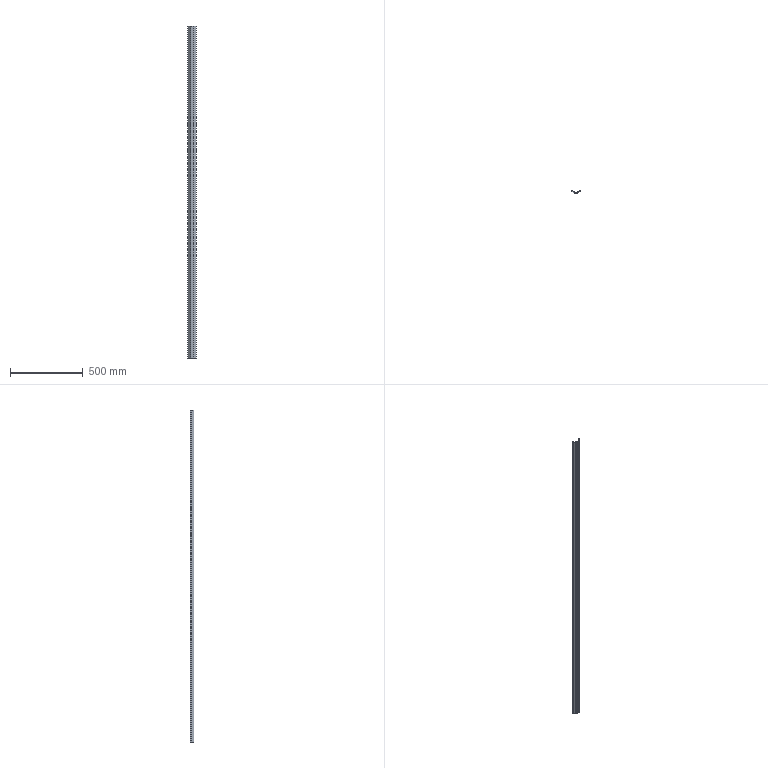Part | SolidWorks | features Extrusion 1 | 1 solid | 40 faces | box 56.572 x 22.358 x 2285 mm | volume 383048 mm3 | plane 37 | cylinder 3 | commonest cylinder face diameters 1 x2 0.5 x1
STEP:
#1=CARTESIAN_POINT('',(6.75,2.,-1142.5));
#2=VERTEX_POINT('',#1);
#3=CARTESIAN_POINT('',(6.75,5.,-1142.5));
#4=VERTEX_POINT('',#3);
#5=CARTESIAN_POINT('',(6.75,2.,-1142.5));
#6=DIRECTION('',(0.,1.,0.));
#7=VECTOR('',#6,1000.);
#8=LINE('',#5,#7);
#9=EDGE_CURVE('',#2,#4,#8,.T.);
#10=ORIENTED_EDGE('',*,*,#9,.T.);
#11=CARTESIAN_POINT('',(6.75,5.,1142.5));
#12=VERTEX_POINT('',#11);
#13=CARTESIAN_POINT('',(6.75,5.,1142.5));
#14=DIRECTION('',(0.,0.,-1.));
#15=VECTOR('',#14,1000.);
#16=LINE('',#13,#15);
#17=EDGE_CURVE('',#12,#4,#16,.T.);
#18=ORIENTED_EDGE('',*,*,#17,.F.);
#19=CARTESIAN_POINT('',(6.75,2.,1142.5));
#20=VERTEX_POINT('',#19);
#21=CARTESIAN_POINT('',(6.75,2.,1142.5));
#22=DIRECTION('',(0.,1.,0.));
#23=VECTOR('',#22,1000.);
#24=LINE('',#21,#23);
#25=EDGE_CURVE('',#20,#12,#24,.T.);
#26=ORIENTED_EDGE('',*,*,#25,.F.);
#27=CARTESIAN_POINT('',(6.75,2.,1142.5));
#28=DIRECTION('',(0.,0.,-1.));
#29=VECTOR('',#28,1000.);
#30=LINE('',#27,#29);
#31=EDGE_CURVE('',#20,#2,#30,.T.);
#32=ORIENTED_EDGE('',*,*,#31,.T.);
#33=EDGE_LOOP('',(#10,#18,#26,#32));
#34=FACE_OUTER_BOUND('',#33,.T.);
#35=CARTESIAN_POINT('',(6.75,2.,1142.5));
#36=DIRECTION('',(-1.,0.,0.));
#37=DIRECTION('',(0.,0.,1.));
#38=AXIS2_PLACEMENT_3D('',#35,#36,#37);
#39=PLANE('',#38);
#40=ADVANCED_FACE('',(#34),#39,.F.);
#41=CARTESIAN_POINT('',(5.25,5.,-1142.5));
#42=VERTEX_POINT('',#41);
#43=CARTESIAN_POINT('',(6.75,5.,-1142.5));
#44=DIRECTION('',(-1.,0.,0.));
#45=VECTOR('',#44,1000.);
#46=LINE('',#43,#45);
#47=EDGE_CURVE('',#4,#42,#46,.T.);
#48=ORIENTED_EDGE('',*,*,#47,.T.);
#49=CARTESIAN_POINT('',(5.25,5.,1142.5));
#50=VERTEX_POINT('',#49);
#51=CARTESIAN_POINT('',(5.25,5.,1142.5));
#52=DIRECTION('',(0.,0.,-1.));
#53=VECTOR('',#52,1000.);
#54=LINE('',#51,#53);
#55=EDGE_CURVE('',#50,#42,#54,.T.);
#56=ORIENTED_EDGE('',*,*,#55,.F.);
#57=CARTESIAN_POINT('',(6.75,5.,1142.5));
#58=DIRECTION('',(-1.,0.,0.));
#59=VECTOR('',#58,1000.);
#60=LINE('',#57,#59);
#61=EDGE_CURVE('',#12,#50,#60,.T.);
#62=ORIENTED_EDGE('',*,*,#61,.F.);
#63=ORIENTED_EDGE('',*,*,#17,.T.);
#64=EDGE_LOOP('',(#48,#56,#62,#63));
#65=FACE_OUTER_BOUND('',#64,.T.);
#66=CARTESIAN_POINT('',(6.75,5.,1142.5));
#67=DIRECTION('',(0.,-1.,0.));
#68=DIRECTION('',(1.,0.,0.));
#69=AXIS2_PLACEMENT_3D('',#66,#67,#68);
#70=PLANE('',#69);
#71=ADVANCED_FACE('',(#65),#70,.F.);
#72=CARTESIAN_POINT('',(5.25,2.,-1142.5));
#73=VERTEX_POINT('',#72);
#74=CARTESIAN_POINT('',(5.25,5.,-1142.5));
#75=DIRECTION('',(0.,-1.,0.));
#76=VECTOR('',#75,1000.);
#77=LINE('',#74,#76);
#78=EDGE_CURVE('',#42,#73,#77,.T.);
#79=ORIENTED_EDGE('',*,*,#78,.T.);
#80=CARTESIAN_POINT('',(5.25,2.,1142.5));
#81=VERTEX_POINT('',#80);
#82=CARTESIAN_POINT('',(5.25,2.,1142.5));
#83=DIRECTION('',(0.,0.,-1.));
#84=VECTOR('',#83,1000.);
#85=LINE('',#82,#84);
#86=EDGE_CURVE('',#81,#73,#85,.T.);
#87=ORIENTED_EDGE('',*,*,#86,.F.);
#88=CARTESIAN_POINT('',(5.25,5.,1142.5));
#89=DIRECTION('',(0.,-1.,0.));
#90=VECTOR('',#89,1000.);
#91=LINE('',#88,#90);
#92=EDGE_CURVE('',#50,#81,#91,.T.);
#93=ORIENTED_EDGE('',*,*,#92,.F.);
#94=ORIENTED_EDGE('',*,*,#55,.T.);
#95=EDGE_LOOP('',(#79,#87,#93,#94));
#96=FACE_OUTER_BOUND('',#95,.T.);
#97=CARTESIAN_POINT('',(5.25,5.,1142.5));
#98=DIRECTION('',(1.,0.,0.));
#99=DIRECTION('',(0.,0.,-1.));
#100=AXIS2_PLACEMENT_3D('',#97,#98,#99);
#101=PLANE('',#100);
#102=ADVANCED_FACE('',(#96),#101,.F.);
#103=CARTESIAN_POINT('',(0.25,2.,-1142.5));
#104=VERTEX_POINT('',#103);
#105=CARTESIAN_POINT('',(5.25,2.,-1142.5));
#106=DIRECTION('',(-1.,0.,0.));
#107=VECTOR('',#106,1000.);
#108=LINE('',#105,#107);
#109=EDGE_CURVE('',#73,#104,#108,.T.);
#110=ORIENTED_EDGE('',*,*,#109,.T.);
#111=CARTESIAN_POINT('',(0.25,2.,1142.5));
#112=VERTEX_POINT('',#111);
#113=CARTESIAN_POINT('',(0.25,2.,1142.5));
#114=DIRECTION('',(0.,0.,-1.));
#115=VECTOR('',#114,1000.);
#116=LINE('',#113,#115);
#117=EDGE_CURVE('',#112,#104,#116,.T.);
#118=ORIENTED_EDGE('',*,*,#117,.F.);
#119=CARTESIAN_POINT('',(5.25,2.,1142.5));
#120=DIRECTION('',(-1.,0.,0.));
#121=VECTOR('',#120,1000.);
#122=LINE('',#119,#121);
#123=EDGE_CURVE('',#81,#112,#122,.T.);
#124=ORIENTED_EDGE('',*,*,#123,.F.);
#125=ORIENTED_EDGE('',*,*,#86,.T.);
#126=EDGE_LOOP('',(#110,#118,#124,#125));
#127=FACE_OUTER_BOUND('',#126,.T.);
#128=CARTESIAN_POINT('',(5.25,2.,1142.5));
#129=DIRECTION('',(0.,-1.,0.));
#130=DIRECTION('',(0.,0.,-1.));
#131=AXIS2_PLACEMENT_3D('',#128,#129,#130);
#132=PLANE('',#131);
#133=ADVANCED_FACE('',(#127),#132,.F.);
#134=CARTESIAN_POINT('',(-0.25,2.,-1142.5));
#135=VERTEX_POINT('',#134);
#136=CARTESIAN_POINT('',(0.,2.,-1142.5));
#137=DIRECTION('',(0.,0.,-1.));
#138=DIRECTION('',(1.,0.,0.));
#139=AXIS2_PLACEMENT_3D('',#136,#137,#138);
#140=CIRCLE('',#139,0.25);
#141=EDGE_CURVE('',#104,#135,#140,.T.);
#142=ORIENTED_EDGE('',*,*,#141,.T.);
#143=CARTESIAN_POINT('',(-0.25,2.,1142.5));
#144=VERTEX_POINT('',#143);
#145=CARTESIAN_POINT('',(-0.25,2.,1142.5));
#146=DIRECTION('',(0.,0.,-1.));
#147=VECTOR('',#146,1000.);
#148=LINE('',#145,#147);
#149=EDGE_CURVE('',#144,#135,#148,.T.);
#150=ORIENTED_EDGE('',*,*,#149,.F.);
#151=CARTESIAN_POINT('',(0.,2.,1142.5));
#152=DIRECTION('',(0.,0.,-1.));
#153=DIRECTION('',(1.,0.,0.));
#154=AXIS2_PLACEMENT_3D('',#151,#152,#153);
#155=CIRCLE('',#154,0.25);
#156=EDGE_CURVE('',#112,#144,#155,.T.);
#157=ORIENTED_EDGE('',*,*,#156,.F.);
#158=ORIENTED_EDGE('',*,*,#117,.T.);
#159=EDGE_LOOP('',(#142,#150,#157,#158));
#160=FACE_OUTER_BOUND('',#159,.T.);
#161=CARTESIAN_POINT('',(0.,2.,1142.5));
#162=DIRECTION('',(0.,0.,-1.));
#163=DIRECTION('',(-1.,0.,0.));
#164=AXIS2_PLACEMENT_3D('',#161,#162,#163);
#165=CYLINDRICAL_SURFACE('',#164,0.25);
#166=ADVANCED_FACE('',(#160),#165,.F.);
#167=CARTESIAN_POINT('',(-5.25,2.,-1142.5));
#168=VERTEX_POINT('',#167);
#169=CARTESIAN_POINT('',(-0.25,2.,-1142.5));
#170=DIRECTION('',(-1.,0.,0.));
#171=VECTOR('',#170,1000.);
#172=LINE('',#169,#171);
#173=EDGE_CURVE('',#135,#168,#172,.T.);
#174=ORIENTED_EDGE('',*,*,#173,.T.);
#175=CARTESIAN_POINT('',(-5.25,2.,1142.5));
#176=VERTEX_POINT('',#175);
#177=CARTESIAN_POINT('',(-5.25,2.,1142.5));
#178=DIRECTION('',(0.,0.,-1.));
#179=VECTOR('',#178,1000.);
#180=LINE('',#177,#179);
#181=EDGE_CURVE('',#176,#168,#180,.T.);
#182=ORIENTED_EDGE('',*,*,#181,.F.);
#183=CARTESIAN_POINT('',(-0.25,2.,1142.5));
#184=DIRECTION('',(-1.,0.,0.));
#185=VECTOR('',#184,1000.);
#186=LINE('',#183,#185);
#187=EDGE_CURVE('',#144,#176,#186,.T.);
#188=ORIENTED_EDGE('',*,*,#187,.F.);
#189=ORIENTED_EDGE('',*,*,#149,.T.);
#190=EDGE_LOOP('',(#174,#182,#188,#189));
#191=FACE_OUTER_BOUND('',#190,.T.);
#192=CARTESIAN_POINT('',(-0.25,2.,1142.5));
#193=DIRECTION('',(0.,-1.,0.));
#194=DIRECTION('',(1.,0.,0.));
#195=AXIS2_PLACEMENT_3D('',#192,#193,#194);
#196=PLANE('',#195);
#197=ADVANCED_FACE('',(#191),#196,.F.);
#198=CARTESIAN_POINT('',(-5.25,5.,-1142.5));
#199=VERTEX_POINT('',#198);
#200=CARTESIAN_POINT('',(-5.25,2.,-1142.5));
#201=DIRECTION('',(0.,1.,0.));
#202=VECTOR('',#201,1000.);
#203=LINE('',#200,#202);
#204=EDGE_CURVE('',#168,#199,#203,.T.);
#205=ORIENTED_EDGE('',*,*,#204,.T.);
#206=CARTESIAN_POINT('',(-5.25,5.,1142.5));
#207=VERTEX_POINT('',#206);
#208=CARTESIAN_POINT('',(-5.25,5.,1142.5));
#209=DIRECTION('',(0.,0.,-1.));
#210=VECTOR('',#209,1000.);
#211=LINE('',#208,#210);
#212=EDGE_CURVE('',#207,#199,#211,.T.);
#213=ORIENTED_EDGE('',*,*,#212,.F.);
#214=CARTESIAN_POINT('',(-5.25,2.,1142.5));
#215=DIRECTION('',(0.,1.,0.));
#216=VECTOR('',#215,1000.);
#217=LINE('',#214,#216);
#218=EDGE_CURVE('',#176,#207,#217,.T.);
#219=ORIENTED_EDGE('',*,*,#218,.F.);
#220=ORIENTED_EDGE('',*,*,#181,.T.);
#221=EDGE_LOOP('',(#205,#213,#219,#220));
#222=FACE_OUTER_BOUND('',#221,.T.);
#223=CARTESIAN_POINT('',(-5.25,2.,1142.5));
#224=DIRECTION('',(-1.,0.,0.));
#225=DIRECTION('',(0.,0.,1.));
#226=AXIS2_PLACEMENT_3D('',#223,#224,#225);
#227=PLANE('',#226);
#228=ADVANCED_FACE('',(#222),#227,.F.);
#229=CARTESIAN_POINT('',(-6.75,5.,-1142.5));
#230=VERTEX_POINT('',#229);
#231=CARTESIAN_POINT('',(-5.25,5.,-1142.5));
#232=DIRECTION('',(-1.,0.,0.));
#233=VECTOR('',#232,1000.);
#234=LINE('',#231,#233);
#235=EDGE_CURVE('',#199,#230,#234,.T.);
#236=ORIENTED_EDGE('',*,*,#235,.T.);
#237=CARTESIAN_POINT('',(-6.75,5.,1142.5));
#238=VERTEX_POINT('',#237);
#239=CARTESIAN_POINT('',(-6.75,5.,1142.5));
#240=DIRECTION('',(0.,0.,-1.));
#241=VECTOR('',#240,1000.);
#242=LINE('',#239,#241);
#243=EDGE_CURVE('',#238,#230,#242,.T.);
#244=ORIENTED_EDGE('',*,*,#243,.F.);
#245=CARTESIAN_POINT('',(-5.25,5.,1142.5));
#246=DIRECTION('',(-1.,0.,0.));
#247=VECTOR('',#246,1000.);
#248=LINE('',#245,#247);
#249=EDGE_CURVE('',#207,#238,#248,.T.);
#250=ORIENTED_EDGE('',*,*,#249,.F.);
#251=ORIENTED_EDGE('',*,*,#212,.T.);
#252=EDGE_LOOP('',(#236,#244,#250,#251));
#253=FACE_OUTER_BOUND('',#252,.T.);
#254=CARTESIAN_POINT('',(-5.25,5.,1142.5));
#255=DIRECTION('',(0.,-1.,0.));
#256=DIRECTION('',(1.,0.,0.));
#257=AXIS2_PLACEMENT_3D('',#254,#255,#256);
#258=PLANE('',#257);
#259=ADVANCED_FACE('',(#253),#258,.F.);
#260=CARTESIAN_POINT('',(-6.75,2.,-1142.5));
#261=VERTEX_POINT('',#260);
#262=CARTESIAN_POINT('',(-6.75,5.,-1142.5));
#263=DIRECTION('',(0.,-1.,0.));
#264=VECTOR('',#263,1000.);
#265=LINE('',#262,#264);
#266=EDGE_CURVE('',#230,#261,#265,.T.);
#267=ORIENTED_EDGE('',*,*,#266,.T.);
#268=CARTESIAN_POINT('',(-6.75,2.,1142.5));
#269=VERTEX_POINT('',#268);
#270=CARTESIAN_POINT('',(-6.75,2.,1142.5));
#271=DIRECTION('',(0.,0.,-1.));
#272=VECTOR('',#271,1000.);
#273=LINE('',#270,#272);
#274=EDGE_CURVE('',#269,#261,#273,.T.);
#275=ORIENTED_EDGE('',*,*,#274,.F.);
#276=CARTESIAN_POINT('',(-6.75,5.,1142.5));
#277=DIRECTION('',(0.,-1.,0.));
#278=VECTOR('',#277,1000.);
#279=LINE('',#276,#278);
#280=EDGE_CURVE('',#238,#269,#279,.T.);
#281=ORIENTED_EDGE('',*,*,#280,.F.);
#282=ORIENTED_EDGE('',*,*,#243,.T.);
#283=EDGE_LOOP('',(#267,#275,#281,#282));
#284=FACE_OUTER_BOUND('',#283,.T.);
#285=CARTESIAN_POINT('',(-6.75,5.,1142.5));
#286=DIRECTION('',(1.,0.,0.));
#287=DIRECTION('',(0.,0.,-1.));
#288=AXIS2_PLACEMENT_3D('',#285,#286,#287);
#289=PLANE('',#288);
#290=ADVANCED_FACE('',(#284),#289,.F.);
#291=CARTESIAN_POINT('',(-8.635,2.,-1142.5));
#292=VERTEX_POINT('',#291);
#293=CARTESIAN_POINT('',(-6.75,2.,-1142.5));
#294=DIRECTION('',(-1.,0.,0.));
#295=VECTOR('',#294,1000.);
#296=LINE('',#293,#295);
#297=EDGE_CURVE('',#261,#292,#296,.T.);
#298=ORIENTED_EDGE('',*,*,#297,.T.);
#299=CARTESIAN_POINT('',(-8.635,2.,1142.5));
#300=VERTEX_POINT('',#299);
#301=CARTESIAN_POINT('',(-8.635,2.,1142.5));
#302=DIRECTION('',(0.,0.,-1.));
#303=VECTOR('',#302,1000.);
#304=LINE('',#301,#303);
#305=EDGE_CURVE('',#300,#292,#304,.T.);
#306=ORIENTED_EDGE('',*,*,#305,.F.);
#307=CARTESIAN_POINT('',(-6.75,2.,1142.5));
#308=DIRECTION('',(-1.,0.,0.));
#309=VECTOR('',#308,1000.);
#310=LINE('',#307,#309);
#311=EDGE_CURVE('',#269,#300,#310,.T.);
#312=ORIENTED_EDGE('',*,*,#311,.F.);
#313=ORIENTED_EDGE('',*,*,#274,.T.);
#314=EDGE_LOOP('',(#298,#306,#312,#313));
#315=FACE_OUTER_BOUND('',#314,.T.);
#316=CARTESIAN_POINT('',(-6.75,2.,1142.5));
#317=DIRECTION('',(0.,-1.,0.));
#318=DIRECTION('',(1.,0.,0.));
#319=AXIS2_PLACEMENT_3D('',#316,#317,#318);
#320=PLANE('',#319);
#321=ADVANCED_FACE('',(#315),#320,.F.);
#322=CARTESIAN_POINT('',(-11.75,5.119,-1142.5));
#323=VERTEX_POINT('',#322);
#324=CARTESIAN_POINT('',(-8.635,2.,-1142.5));
#325=DIRECTION('',(-0.7067,0.7076,0.));
#326=VECTOR('',#325,1000.);
#327=LINE('',#324,#326);
#328=EDGE_CURVE('',#292,#323,#327,.T.);
#329=ORIENTED_EDGE('',*,*,#328,.T.);
#330=CARTESIAN_POINT('',(-11.75,5.119,1142.5));
#331=VERTEX_POINT('',#330);
#332=CARTESIAN_POINT('',(-11.75,5.119,1142.5));
#333=DIRECTION('',(0.,0.,-1.));
#334=VECTOR('',#333,1000.);
#335=LINE('',#332,#334);
#336=EDGE_CURVE('',#331,#323,#335,.T.);
#337=ORIENTED_EDGE('',*,*,#336,.F.);
#338=CARTESIAN_POINT('',(-8.635,2.,1142.5));
#339=DIRECTION('',(-0.7067,0.7076,0.));
#340=VECTOR('',#339,1000.);
#341=LINE('',#338,#340);
#342=EDGE_CURVE('',#300,#331,#341,.T.);
#343=ORIENTED_EDGE('',*,*,#342,.F.);
#344=ORIENTED_EDGE('',*,*,#305,.T.);
#345=EDGE_LOOP('',(#329,#337,#343,#344));
#346=FACE_OUTER_BOUND('',#345,.T.);
#347=CARTESIAN_POINT('',(-8.635,2.,1142.5));
#348=DIRECTION('',(-0.7076,-0.7067,0.));
#349=DIRECTION('',(0.7067,-0.7076,0.));
#350=AXIS2_PLACEMENT_3D('',#347,#348,#349);
#351=PLANE('',#350);
#352=ADVANCED_FACE('',(#346),#351,.F.);
#353=CARTESIAN_POINT('',(-11.75,8.887,-1142.5));
#354=VERTEX_POINT('',#353);
#355=CARTESIAN_POINT('',(-11.75,5.119,-1142.5));
#356=DIRECTION('',(0.,1.,0.));
#357=VECTOR('',#356,1000.);
#358=LINE('',#355,#357);
#359=EDGE_CURVE('',#323,#354,#358,.T.);
#360=ORIENTED_EDGE('',*,*,#359,.T.);
#361=CARTESIAN_POINT('',(-11.75,8.887,1142.5));
#362=VERTEX_POINT('',#361);
#363=CARTESIAN_POINT('',(-11.75,8.887,1142.5));
#364=DIRECTION('',(0.,0.,-1.));
#365=VECTOR('',#364,1000.);
#366=LINE('',#363,#365);
#367=EDGE_CURVE('',#362,#354,#366,.T.);
#368=ORIENTED_EDGE('',*,*,#367,.F.);
#369=CARTESIAN_POINT('',(-11.75,5.119,1142.5));
#370=DIRECTION('',(0.,1.,0.));
#371=VECTOR('',#370,1000.);
#372=LINE('',#369,#371);
#373=EDGE_CURVE('',#331,#362,#372,.T.);
#374=ORIENTED_EDGE('',*,*,#373,.F.);
#375=ORIENTED_EDGE('',*,*,#336,.T.);
#376=EDGE_LOOP('',(#360,#368,#374,#375));
#377=FACE_OUTER_BOUND('',#376,.T.);
#378=CARTESIAN_POINT('',(-11.75,5.119,1142.5));
#379=DIRECTION('',(-1.,0.,0.));
#380=DIRECTION('',(0.,0.,1.));
#381=AXIS2_PLACEMENT_3D('',#378,#379,#380);
#382=PLANE('',#381);
#383=ADVANCED_FACE('',(#377),#382,.F.);
#384=CARTESIAN_POINT('',(-12.25,9.387,-1142.5));
#385=VERTEX_POINT('',#384);
#386=CARTESIAN_POINT('',(-11.75,8.887,-1142.5));
#387=DIRECTION('',(-0.7071,0.7071,0.));
#388=VECTOR('',#387,1000.);
#389=LINE('',#386,#388);
#390=EDGE_CURVE('',#354,#385,#389,.T.);
#391=ORIENTED_EDGE('',*,*,#390,.T.);
#392=CARTESIAN_POINT('',(-12.25,9.387,1142.5));
#393=VERTEX_POINT('',#392);
#394=CARTESIAN_POINT('',(-12.25,9.387,1142.5));
#395=DIRECTION('',(0.,0.,-1.));
#396=VECTOR('',#395,1000.);
#397=LINE('',#394,#396);
#398=EDGE_CURVE('',#393,#385,#397,.T.);
#399=ORIENTED_EDGE('',*,*,#398,.F.);
#400=CARTESIAN_POINT('',(-11.75,8.887,1142.5));
#401=DIRECTION('',(-0.7071,0.7071,0.));
#402=VECTOR('',#401,1000.);
#403=LINE('',#400,#402);
#404=EDGE_CURVE('',#362,#393,#403,.T.);
#405=ORIENTED_EDGE('',*,*,#404,.F.);
#406=ORIENTED_EDGE('',*,*,#367,.T.);
#407=EDGE_LOOP('',(#391,#399,#405,#406));
#408=FACE_OUTER_BOUND('',#407,.T.);
#409=CARTESIAN_POINT('',(-11.75,8.887,1142.5));
#410=DIRECTION('',(-0.7071,-0.7071,0.));
#411=DIRECTION('',(0.7071,-0.7071,0.));
#412=AXIS2_PLACEMENT_3D('',#409,#410,#411);
#413=PLANE('',#412);
#414=ADVANCED_FACE('',(#408),#413,.F.);
#415=CARTESIAN_POINT('',(-12.75,9.387,-1142.5));
#416=VERTEX_POINT('',#415);
#417=CARTESIAN_POINT('',(-12.25,9.387,-1142.5));
#418=DIRECTION('',(-1.,0.,0.));
#419=VECTOR('',#418,1000.);
#420=LINE('',#417,#419);
#421=EDGE_CURVE('',#385,#416,#420,.T.);
#422=ORIENTED_EDGE('',*,*,#421,.T.);
#423=CARTESIAN_POINT('',(-12.75,9.387,1142.5));
#424=VERTEX_POINT('',#423);
#425=CARTESIAN_POINT('',(-12.75,9.387,1142.5));
#426=DIRECTION('',(0.,0.,-1.));
#427=VECTOR('',#426,1000.);
#428=LINE('',#425,#427);
#429=EDGE_CURVE('',#424,#416,#428,.T.);
#430=ORIENTED_EDGE('',*,*,#429,.F.);
#431=CARTESIAN_POINT('',(-12.25,9.387,1142.5));
#432=DIRECTION('',(-1.,0.,0.));
#433=VECTOR('',#432,1000.);
#434=LINE('',#431,#433);
#435=EDGE_CURVE('',#393,#424,#434,.T.);
#436=ORIENTED_EDGE('',*,*,#435,.F.);
#437=ORIENTED_EDGE('',*,*,#398,.T.);
#438=EDGE_LOOP('',(#422,#430,#436,#437));
#439=FACE_OUTER_BOUND('',#438,.T.);
#440=CARTESIAN_POINT('',(-12.25,9.387,1142.5));
#441=DIRECTION('',(0.,-1.,0.));
#442=DIRECTION('',(0.,0.,-1.));
#443=AXIS2_PLACEMENT_3D('',#440,#441,#442);
#444=PLANE('',#443);
#445=ADVANCED_FACE('',(#439),#444,.F.);
#446=CARTESIAN_POINT('',(-12.75,7.328,-1142.5));
#447=VERTEX_POINT('',#446);
#448=CARTESIAN_POINT('',(-12.75,9.387,-1142.5));
#449=DIRECTION('',(0.,-1.,0.));
#450=VECTOR('',#449,1000.);
#451=LINE('',#448,#450);
#452=EDGE_CURVE('',#416,#447,#451,.T.);
#453=ORIENTED_EDGE('',*,*,#452,.T.);
#454=CARTESIAN_POINT('',(-12.75,7.328,1142.5));
#455=VERTEX_POINT('',#454);
#456=CARTESIAN_POINT('',(-12.75,7.328,1142.5));
#457=DIRECTION('',(0.,0.,-1.));
#458=VECTOR('',#457,1000.);
#459=LINE('',#456,#458);
#460=EDGE_CURVE('',#455,#447,#459,.T.);
#461=ORIENTED_EDGE('',*,*,#460,.F.);
#462=CARTESIAN_POINT('',(-12.75,9.387,1142.5));
#463=DIRECTION('',(0.,-1.,0.));
#464=VECTOR('',#463,1000.);
#465=LINE('',#462,#464);
#466=EDGE_CURVE('',#424,#455,#465,.T.);
#467=ORIENTED_EDGE('',*,*,#466,.F.);
#468=ORIENTED_EDGE('',*,*,#429,.T.);
#469=EDGE_LOOP('',(#453,#461,#467,#468));
#470=FACE_OUTER_BOUND('',#469,.T.);
#471=CARTESIAN_POINT('',(-12.75,9.387,1142.5));
#472=DIRECTION('',(1.,0.,0.));
#473=DIRECTION('',(0.,0.,-1.));
#474=AXIS2_PLACEMENT_3D('',#471,#472,#473);
#475=PLANE('',#474);
#476=ADVANCED_FACE('',(#470),#475,.F.);
#477=CARTESIAN_POINT('',(-13.604,6.975,-1142.5));
#478=VERTEX_POINT('',#477);
#479=CARTESIAN_POINT('',(-13.25,7.328,-1142.5));
#480=DIRECTION('',(0.,0.,-1.));
#481=DIRECTION('',(1.,0.,0.));
#482=AXIS2_PLACEMENT_3D('',#479,#480,#481);
#483=CIRCLE('',#482,0.5);
#484=EDGE_CURVE('',#447,#478,#483,.T.);
#485=ORIENTED_EDGE('',*,*,#484,.T.);
#486=CARTESIAN_POINT('',(-13.604,6.975,1142.5));
#487=VERTEX_POINT('',#486);
#488=CARTESIAN_POINT('',(-13.604,6.975,1142.5));
#489=DIRECTION('',(0.,0.,-1.));
#490=VECTOR('',#489,1000.);
#491=LINE('',#488,#490);
#492=EDGE_CURVE('',#487,#478,#491,.T.);
#493=ORIENTED_EDGE('',*,*,#492,.F.);
#494=CARTESIAN_POINT('',(-13.25,7.328,1142.5));
#495=DIRECTION('',(0.,0.,-1.));
#496=DIRECTION('',(1.,0.,0.));
#497=AXIS2_PLACEMENT_3D('',#494,#495,#496);
#498=CIRCLE('',#497,0.5);
#499=EDGE_CURVE('',#455,#487,#498,.T.);
#500=ORIENTED_EDGE('',*,*,#499,.F.);
#501=ORIENTED_EDGE('',*,*,#460,.T.);
#502=EDGE_LOOP('',(#485,#493,#500,#501));
#503=FACE_OUTER_BOUND('',#502,.T.);
#504=CARTESIAN_POINT('',(-13.25,7.328,1142.5));
#505=DIRECTION('',(0.,0.,-1.));
#506=DIRECTION('',(-1.,0.,0.));
#507=AXIS2_PLACEMENT_3D('',#504,#505,#506);
#508=CYLINDRICAL_SURFACE('',#507,0.5);
#509=ADVANCED_FACE('',(#503),#508,.F.);
#510=CARTESIAN_POINT('',(-23.891,17.282,-1142.5));
#511=VERTEX_POINT('',#510);
#512=CARTESIAN_POINT('',(-13.604,6.975,-1142.5));
#513=DIRECTION('',(-0.7064,0.7078,0.));
#514=VECTOR('',#513,1000.);
#515=LINE('',#512,#514);
#516=EDGE_CURVE('',#478,#511,#515,.T.);
#517=ORIENTED_EDGE('',*,*,#516,.T.);
#518=CARTESIAN_POINT('',(-23.891,17.282,1142.5));
#519=VERTEX_POINT('',#518);
#520=CARTESIAN_POINT('',(-23.891,17.282,1142.5));
#521=DIRECTION('',(0.,0.,-1.));
#522=VECTOR('',#521,1000.);
#523=LINE('',#520,#522);
#524=EDGE_CURVE('',#519,#511,#523,.T.);
#525=ORIENTED_EDGE('',*,*,#524,.F.);
#526=CARTESIAN_POINT('',(-13.604,6.975,1142.5));
#527=DIRECTION('',(-0.7064,0.7078,0.));
#528=VECTOR('',#527,1000.);
#529=LINE('',#526,#528);
#530=EDGE_CURVE('',#487,#519,#529,.T.);
#531=ORIENTED_EDGE('',*,*,#530,.F.);
#532=ORIENTED_EDGE('',*,*,#492,.T.);
#533=EDGE_LOOP('',(#517,#525,#531,#532));
#534=FACE_OUTER_BOUND('',#533,.T.);
#535=CARTESIAN_POINT('',(-13.604,6.975,1142.5));
#536=DIRECTION('',(-0.7078,-0.7064,0.));
#537=DIRECTION('',(0.7064,-0.7078,0.));
#538=AXIS2_PLACEMENT_3D('',#535,#536,#537);
#539=PLANE('',#538);
#540=ADVANCED_FACE('',(#534),#539,.F.);
#541=CARTESIAN_POINT('',(-23.891,19.376,-1142.5));
#542=VERTEX_POINT('',#541);
#543=CARTESIAN_POINT('',(-23.891,17.282,-1142.5));
#544=DIRECTION('',(0.,1.,0.));
#545=VECTOR('',#544,1000.);
#546=LINE('',#543,#545);
#547=EDGE_CURVE('',#511,#542,#546,.T.);
#548=ORIENTED_EDGE('',*,*,#547,.T.);
#549=CARTESIAN_POINT('',(-23.891,19.376,1142.5));
#550=VERTEX_POINT('',#549);
#551=CARTESIAN_POINT('',(-23.891,19.376,1142.5));
#552=DIRECTION('',(0.,0.,-1.));
#553=VECTOR('',#552,1000.);
#554=LINE('',#551,#553);
#555=EDGE_CURVE('',#550,#542,#554,.T.);
#556=ORIENTED_EDGE('',*,*,#555,.F.);
#557=CARTESIAN_POINT('',(-23.891,17.282,1142.5));
#558=DIRECTION('',(0.,1.,0.));
#559=VECTOR('',#558,1000.);
#560=LINE('',#557,#559);
#561=EDGE_CURVE('',#519,#550,#560,.T.);
#562=ORIENTED_EDGE('',*,*,#561,.F.);
#563=ORIENTED_EDGE('',*,*,#524,.T.);
#564=EDGE_LOOP('',(#548,#556,#562,#563));
#565=FACE_OUTER_BOUND('',#564,.T.);
#566=CARTESIAN_POINT('',(-23.891,17.282,1142.5));
#567=DIRECTION('',(-1.,0.,0.));
#568=DIRECTION('',(0.,0.,1.));
#569=AXIS2_PLACEMENT_3D('',#566,#567,#568);
#570=PLANE('',#569);
#571=ADVANCED_FACE('',(#565),#570,.F.);
#572=CARTESIAN_POINT('',(-26.873,22.358,-1142.5));
#573=VERTEX_POINT('',#572);
#574=CARTESIAN_POINT('',(-23.891,19.376,-1142.5));
#575=DIRECTION('',(-0.7071,0.7071,0.));
#576=VECTOR('',#575,1000.);
#577=LINE('',#574,#576);
#578=EDGE_CURVE('',#542,#573,#577,.T.);
#579=ORIENTED_EDGE('',*,*,#578,.T.);
#580=CARTESIAN_POINT('',(-26.873,22.358,1142.5));
#581=VERTEX_POINT('',#580);
#582=CARTESIAN_POINT('',(-26.873,22.358,1142.5));
#583=DIRECTION('',(0.,0.,-1.));
#584=VECTOR('',#583,1000.);
#585=LINE('',#582,#584);
#586=EDGE_CURVE('',#581,#573,#585,.T.);
#587=ORIENTED_EDGE('',*,*,#586,.F.);
#588=CARTESIAN_POINT('',(-23.891,19.376,1142.5));
#589=DIRECTION('',(-0.7071,0.7071,0.));
#590=VECTOR('',#589,1000.);
#591=LINE('',#588,#590);
#592=EDGE_CURVE('',#550,#581,#591,.T.);
#593=ORIENTED_EDGE('',*,*,#592,.F.);
#594=ORIENTED_EDGE('',*,*,#555,.T.);
#595=EDGE_LOOP('',(#579,#587,#593,#594));
#596=FACE_OUTER_BOUND('',#595,.T.);
#597=CARTESIAN_POINT('',(-23.891,19.376,1142.5));
#598=DIRECTION('',(-0.7071,-0.7071,0.));
#599=DIRECTION('',(0.7071,-0.7071,0.));
#600=AXIS2_PLACEMENT_3D('',#597,#598,#599);
#601=PLANE('',#600);
#602=ADVANCED_FACE('',(#596),#601,.F.);
#603=CARTESIAN_POINT('',(-27.58,22.358,-1142.5));
#604=VERTEX_POINT('',#603);
#605=CARTESIAN_POINT('',(-26.873,22.358,-1142.5));
#606=DIRECTION('',(-1.,0.,0.));
#607=VECTOR('',#606,1000.);
#608=LINE('',#605,#607);
#609=EDGE_CURVE('',#573,#604,#608,.T.);
#610=ORIENTED_EDGE('',*,*,#609,.T.);
#611=CARTESIAN_POINT('',(-27.58,22.358,1142.5));
#612=VERTEX_POINT('',#611);
#613=CARTESIAN_POINT('',(-27.58,22.358,1142.5));
#614=DIRECTION('',(0.,0.,-1.));
#615=VECTOR('',#614,1000.);
#616=LINE('',#613,#615);
#617=EDGE_CURVE('',#612,#604,#616,.T.);
#618=ORIENTED_EDGE('',*,*,#617,.F.);
#619=CARTESIAN_POINT('',(-26.873,22.358,1142.5));
#620=DIRECTION('',(-1.,0.,0.));
#621=VECTOR('',#620,1000.);
#622=LINE('',#619,#621);
#623=EDGE_CURVE('',#581,#612,#622,.T.);
#624=ORIENTED_EDGE('',*,*,#623,.F.);
#625=ORIENTED_EDGE('',*,*,#586,.T.);
#626=EDGE_LOOP('',(#610,#618,#624,#625));
#627=FACE_OUTER_BOUND('',#626,.T.);
#628=CARTESIAN_POINT('',(-26.873,22.358,1142.5));
#629=DIRECTION('',(0.,-1.,0.));
#630=DIRECTION('',(0.,0.,-1.));
#631=AXIS2_PLACEMENT_3D('',#628,#629,#630);
#632=PLANE('',#631);
#633=ADVANCED_FACE('',(#627),#632,.F.);
#634=CARTESIAN_POINT('',(-28.284,21.654,-1142.5));
#635=VERTEX_POINT('',#634);
#636=CARTESIAN_POINT('',(-27.58,22.358,-1142.5));
#637=DIRECTION('',(-0.7071,-0.7071,0.));
#638=VECTOR('',#637,1000.);
#639=LINE('',#636,#638);
#640=EDGE_CURVE('',#604,#635,#639,.T.);
#641=ORIENTED_EDGE('',*,*,#640,.T.);
#642=CARTESIAN_POINT('',(-28.284,21.654,1142.5));
#643=VERTEX_POINT('',#642);
#644=CARTESIAN_POINT('',(-28.284,21.654,1142.5));
#645=DIRECTION('',(0.,0.,-1.));
#646=VECTOR('',#645,1000.);
#647=LINE('',#644,#646);
#648=EDGE_CURVE('',#643,#635,#647,.T.);
#649=ORIENTED_EDGE('',*,*,#648,.F.);
#650=CARTESIAN_POINT('',(-27.58,22.358,1142.5));
#651=DIRECTION('',(-0.7071,-0.7071,0.));
#652=VECTOR('',#651,1000.);
#653=LINE('',#650,#652);
#654=EDGE_CURVE('',#612,#643,#653,.T.);
#655=ORIENTED_EDGE('',*,*,#654,.F.);
#656=ORIENTED_EDGE('',*,*,#617,.T.);
#657=EDGE_LOOP('',(#641,#649,#655,#656));
#658=FACE_OUTER_BOUND('',#657,.T.);
#659=CARTESIAN_POINT('',(-27.58,22.358,1142.5));
#660=DIRECTION('',(0.7071,-0.7071,0.));
#661=DIRECTION('',(0.7071,0.7071,0.));
#662=AXIS2_PLACEMENT_3D('',#659,#660,#661);
#663=PLANE('',#662);
#664=ADVANCED_FACE('',(#658),#663,.F.);
#665=CARTESIAN_POINT('',(-28.284,19.103,-1142.5));
#666=VERTEX_POINT('',#665);
#667=CARTESIAN_POINT('',(-28.284,21.654,-1142.5));
#668=DIRECTION('',(0.,-1.,0.));
#669=VECTOR('',#668,1000.);
#670=LINE('',#667,#669);
#671=EDGE_CURVE('',#635,#666,#670,.T.);
#672=ORIENTED_EDGE('',*,*,#671,.T.);
#673=CARTESIAN_POINT('',(-28.284,19.103,1142.5));
#674=VERTEX_POINT('',#673);
#675=CARTESIAN_POINT('',(-28.284,19.103,1142.5));
#676=DIRECTION('',(0.,0.,-1.));
#677=VECTOR('',#676,1000.);
#678=LINE('',#675,#677);
#679=EDGE_CURVE('',#674,#666,#678,.T.);
#680=ORIENTED_EDGE('',*,*,#679,.F.);
#681=CARTESIAN_POINT('',(-28.284,21.654,1142.5));
#682=DIRECTION('',(0.,-1.,0.));
#683=VECTOR('',#682,1000.);
#684=LINE('',#681,#683);
#685=EDGE_CURVE('',#643,#674,#684,.T.);
#686=ORIENTED_EDGE('',*,*,#685,.F.);
#687=ORIENTED_EDGE('',*,*,#648,.T.);
#688=EDGE_LOOP('',(#672,#680,#686,#687));
#689=FACE_OUTER_BOUND('',#688,.T.);
#690=CARTESIAN_POINT('',(-28.284,21.654,1142.5));
#691=DIRECTION('',(1.,0.,0.));
#692=DIRECTION('',(0.,0.,-1.));
#693=AXIS2_PLACEMENT_3D('',#690,#691,#692);
#694=PLANE('',#693);
#695=ADVANCED_FACE('',(#689),#694,.F.);
#696=CARTESIAN_POINT('',(-9.182,0.,-1142.5));
#697=VERTEX_POINT('',#696);
#698=CARTESIAN_POINT('',(-28.284,19.103,-1142.5));
#699=DIRECTION('',(0.7071,-0.7071,0.));
#700=VECTOR('',#699,1000.);
#701=LINE('',#698,#700);
#702=EDGE_CURVE('',#666,#697,#701,.T.);
#703=ORIENTED_EDGE('',*,*,#702,.T.);
#704=CARTESIAN_POINT('',(-9.182,0.,1142.5));
#705=VERTEX_POINT('',#704);
#706=CARTESIAN_POINT('',(-9.182,0.,1142.5));
#707=DIRECTION('',(0.,0.,-1.));
#708=VECTOR('',#707,1000.);
#709=LINE('',#706,#708);
#710=EDGE_CURVE('',#705,#697,#709,.T.);
#711=ORIENTED_EDGE('',*,*,#710,.F.);
#712=CARTESIAN_POINT('',(-28.284,19.103,1142.5));
#713=DIRECTION('',(0.7071,-0.7071,0.));
#714=VECTOR('',#713,1000.);
#715=LINE('',#712,#714);
#716=EDGE_CURVE('',#674,#705,#715,.T.);
#717=ORIENTED_EDGE('',*,*,#716,.F.);
#718=ORIENTED_EDGE('',*,*,#679,.T.);
#719=EDGE_LOOP('',(#703,#711,#717,#718));
#720=FACE_OUTER_BOUND('',#719,.T.);
#721=CARTESIAN_POINT('',(-28.284,19.103,1142.5));
#722=DIRECTION('',(0.7071,0.7071,0.));
#723=DIRECTION('',(-0.7071,0.7071,0.));
#724=AXIS2_PLACEMENT_3D('',#721,#722,#723);
#725=PLANE('',#724);
#726=ADVANCED_FACE('',(#720),#725,.F.);
#727=CARTESIAN_POINT('',(9.182,0.,-1142.5));
#728=VERTEX_POINT('',#727);
#729=CARTESIAN_POINT('',(-9.182,0.,-1142.5));
#730=DIRECTION('',(1.,0.,0.));
#731=VECTOR('',#730,1000.);
#732=LINE('',#729,#731);
#733=EDGE_CURVE('',#697,#728,#732,.T.);
#734=ORIENTED_EDGE('',*,*,#733,.T.);
#735=CARTESIAN_POINT('',(9.182,0.,1142.5));
#736=VERTEX_POINT('',#735);
#737=CARTESIAN_POINT('',(9.182,0.,1142.5));
#738=DIRECTION('',(0.,0.,-1.));
#739=VECTOR('',#738,1000.);
#740=LINE('',#737,#739);
#741=EDGE_CURVE('',#736,#728,#740,.T.);
#742=ORIENTED_EDGE('',*,*,#741,.F.);
#743=CARTESIAN_POINT('',(-9.182,0.,1142.5));
#744=DIRECTION('',(1.,0.,0.));
#745=VECTOR('',#744,1000.);
#746=LINE('',#743,#745);
#747=EDGE_CURVE('',#705,#736,#746,.T.);
#748=ORIENTED_EDGE('',*,*,#747,.F.);
#749=ORIENTED_EDGE('',*,*,#710,.T.);
#750=EDGE_LOOP('',(#734,#742,#748,#749));
#751=FACE_OUTER_BOUND('',#750,.T.);
#752=CARTESIAN_POINT('',(-9.182,0.,1142.5));
#753=DIRECTION('',(0.,1.,0.));
#754=DIRECTION('',(-1.,0.,0.));
#755=AXIS2_PLACEMENT_3D('',#752,#753,#754);
#756=PLANE('',#755);
#757=ADVANCED_FACE('',(#751),#756,.F.);
#758=CARTESIAN_POINT('',(28.287,19.106,-1142.5));
#759=VERTEX_POINT('',#758);
#760=CARTESIAN_POINT('',(9.182,0.,-1142.5));
#761=DIRECTION('',(0.7071,0.7071,0.));
#762=VECTOR('',#761,1000.);
#763=LINE('',#760,#762);
#764=EDGE_CURVE('',#728,#759,#763,.T.);
#765=ORIENTED_EDGE('',*,*,#764,.T.);
#766=CARTESIAN_POINT('',(28.287,19.106,1142.5));
#767=VERTEX_POINT('',#766);
#768=CARTESIAN_POINT('',(28.287,19.106,1142.5));
#769=DIRECTION('',(0.,0.,-1.));
#770=VECTOR('',#769,1000.);
#771=LINE('',#768,#770);
#772=EDGE_CURVE('',#767,#759,#771,.T.);
#773=ORIENTED_EDGE('',*,*,#772,.F.);
#774=CARTESIAN_POINT('',(9.182,0.,1142.5));
#775=DIRECTION('',(0.7071,0.7071,0.));
#776=VECTOR('',#775,1000.);
#777=LINE('',#774,#776);
#778=EDGE_CURVE('',#736,#767,#777,.T.);
#779=ORIENTED_EDGE('',*,*,#778,.F.);
#780=ORIENTED_EDGE('',*,*,#741,.T.);
#781=EDGE_LOOP('',(#765,#773,#779,#780));
#782=FACE_OUTER_BOUND('',#781,.T.);
#783=CARTESIAN_POINT('',(9.182,0.,1142.5));
#784=DIRECTION('',(-0.7071,0.7071,0.));
#785=DIRECTION('',(-0.7071,-0.7071,0.));
#786=AXIS2_PLACEMENT_3D('',#783,#784,#785);
#787=PLANE('',#786);
#788=ADVANCED_FACE('',(#782),#787,.F.);
#789=CARTESIAN_POINT('',(28.287,21.651,-1142.5));
#790=VERTEX_POINT('',#789);
#791=CARTESIAN_POINT('',(28.287,19.106,-1142.5));
#792=DIRECTION('',(0.,1.,0.));
#793=VECTOR('',#792,1000.);
#794=LINE('',#791,#793);
#795=EDGE_CURVE('',#759,#790,#794,.T.);
#796=ORIENTED_EDGE('',*,*,#795,.T.);
#797=CARTESIAN_POINT('',(28.287,21.651,1142.5));
#798=VERTEX_POINT('',#797);
#799=CARTESIAN_POINT('',(28.287,21.651,1142.5));
#800=DIRECTION('',(0.,0.,-1.));
#801=VECTOR('',#800,1000.);
#802=LINE('',#799,#801);
#803=EDGE_CURVE('',#798,#790,#802,.T.);
#804=ORIENTED_EDGE('',*,*,#803,.F.);
#805=CARTESIAN_POINT('',(28.287,19.106,1142.5));
#806=DIRECTION('',(0.,1.,0.));
#807=VECTOR('',#806,1000.);
#808=LINE('',#805,#807);
#809=EDGE_CURVE('',#767,#798,#808,.T.);
#810=ORIENTED_EDGE('',*,*,#809,.F.);
#811=ORIENTED_EDGE('',*,*,#772,.T.);
#812=EDGE_LOOP('',(#796,#804,#810,#811));
#813=FACE_OUTER_BOUND('',#812,.T.);
#814=CARTESIAN_POINT('',(28.287,19.106,1142.5));
#815=DIRECTION('',(-1.,0.,0.));
#816=DIRECTION('',(0.,-1.,0.));
#817=AXIS2_PLACEMENT_3D('',#814,#815,#816);
#818=PLANE('',#817);
#819=ADVANCED_FACE('',(#813),#818,.F.);
#820=CARTESIAN_POINT('',(27.58,22.358,-1142.5));
#821=VERTEX_POINT('',#820);
#822=CARTESIAN_POINT('',(28.287,21.651,-1142.5));
#823=DIRECTION('',(-0.7071,0.7071,0.));
#824=VECTOR('',#823,1000.);
#825=LINE('',#822,#824);
#826=EDGE_CURVE('',#790,#821,#825,.T.);
#827=ORIENTED_EDGE('',*,*,#826,.T.);
#828=CARTESIAN_POINT('',(27.58,22.358,1142.5));
#829=VERTEX_POINT('',#828);
#830=CARTESIAN_POINT('',(27.58,22.358,1142.5));
#831=DIRECTION('',(0.,0.,-1.));
#832=VECTOR('',#831,1000.);
#833=LINE('',#830,#832);
#834=EDGE_CURVE('',#829,#821,#833,.T.);
#835=ORIENTED_EDGE('',*,*,#834,.F.);
#836=CARTESIAN_POINT('',(28.287,21.651,1142.5));
#837=DIRECTION('',(-0.7071,0.7071,0.));
#838=VECTOR('',#837,1000.);
#839=LINE('',#836,#838);
#840=EDGE_CURVE('',#798,#829,#839,.T.);
#841=ORIENTED_EDGE('',*,*,#840,.F.);
#842=ORIENTED_EDGE('',*,*,#803,.T.);
#843=EDGE_LOOP('',(#827,#835,#841,#842));
#844=FACE_OUTER_BOUND('',#843,.T.);
#845=CARTESIAN_POINT('',(28.287,21.651,1142.5));
#846=DIRECTION('',(-0.7071,-0.7071,0.));
#847=DIRECTION('',(0.7071,-0.7071,0.));
#848=AXIS2_PLACEMENT_3D('',#845,#846,#847);
#849=PLANE('',#848);
#850=ADVANCED_FACE('',(#844),#849,.F.);
#851=CARTESIAN_POINT('',(26.873,22.358,-1142.5));
#852=VERTEX_POINT('',#851);
#853=CARTESIAN_POINT('',(27.58,22.358,-1142.5));
#854=DIRECTION('',(-1.,0.,0.));
#855=VECTOR('',#854,1000.);
#856=LINE('',#853,#855);
#857=EDGE_CURVE('',#821,#852,#856,.T.);
#858=ORIENTED_EDGE('',*,*,#857,.T.);
#859=CARTESIAN_POINT('',(26.873,22.358,1142.5));
#860=VERTEX_POINT('',#859);
#861=CARTESIAN_POINT('',(26.873,22.358,1142.5));
#862=DIRECTION('',(0.,0.,-1.));
#863=VECTOR('',#862,1000.);
#864=LINE('',#861,#863);
#865=EDGE_CURVE('',#860,#852,#864,.T.);
#866=ORIENTED_EDGE('',*,*,#865,.F.);
#867=CARTESIAN_POINT('',(27.58,22.358,1142.5));
#868=DIRECTION('',(-1.,0.,0.));
#869=VECTOR('',#868,1000.);
#870=LINE('',#867,#869);
#871=EDGE_CURVE('',#829,#860,#870,.T.);
#872=ORIENTED_EDGE('',*,*,#871,.F.);
#873=ORIENTED_EDGE('',*,*,#834,.T.);
#874=EDGE_LOOP('',(#858,#866,#872,#873));
#875=FACE_OUTER_BOUND('',#874,.T.);
#876=CARTESIAN_POINT('',(27.58,22.358,1142.5));
#877=DIRECTION('',(0.,-1.,0.));
#878=DIRECTION('',(1.,0.,0.));
#879=AXIS2_PLACEMENT_3D('',#876,#877,#878);
#880=PLANE('',#879);
#881=ADVANCED_FACE('',(#875),#880,.F.);
#882=CARTESIAN_POINT('',(23.891,19.376,-1142.5));
#883=VERTEX_POINT('',#882);
#884=CARTESIAN_POINT('',(26.873,22.358,-1142.5));
#885=DIRECTION('',(-0.7071,-0.7071,0.));
#886=VECTOR('',#885,1000.);
#887=LINE('',#884,#886);
#888=EDGE_CURVE('',#852,#883,#887,.T.);
#889=ORIENTED_EDGE('',*,*,#888,.T.);
#890=CARTESIAN_POINT('',(23.891,19.376,1142.5));
#891=VERTEX_POINT('',#890);
#892=CARTESIAN_POINT('',(23.891,19.376,1142.5));
#893=DIRECTION('',(0.,0.,-1.));
#894=VECTOR('',#893,1000.);
#895=LINE('',#892,#894);
#896=EDGE_CURVE('',#891,#883,#895,.T.);
#897=ORIENTED_EDGE('',*,*,#896,.F.);
#898=CARTESIAN_POINT('',(26.873,22.358,1142.5));
#899=DIRECTION('',(-0.7071,-0.7071,0.));
#900=VECTOR('',#899,1000.);
#901=LINE('',#898,#900);
#902=EDGE_CURVE('',#860,#891,#901,.T.);
#903=ORIENTED_EDGE('',*,*,#902,.F.);
#904=ORIENTED_EDGE('',*,*,#865,.T.);
#905=EDGE_LOOP('',(#889,#897,#903,#904));
#906=FACE_OUTER_BOUND('',#905,.T.);
#907=CARTESIAN_POINT('',(26.873,22.358,1142.5));
#908=DIRECTION('',(0.7071,-0.7071,0.));
#909=DIRECTION('',(0.7071,0.7071,0.));
#910=AXIS2_PLACEMENT_3D('',#907,#908,#909);
#911=PLANE('',#910);
#912=ADVANCED_FACE('',(#906),#911,.F.);
#913=CARTESIAN_POINT('',(23.891,17.282,-1142.5));
#914=VERTEX_POINT('',#913);
#915=CARTESIAN_POINT('',(23.891,19.376,-1142.5));
#916=DIRECTION('',(0.,-1.,0.));
#917=VECTOR('',#916,1000.);
#918=LINE('',#915,#917);
#919=EDGE_CURVE('',#883,#914,#918,.T.);
#920=ORIENTED_EDGE('',*,*,#919,.T.);
#921=CARTESIAN_POINT('',(23.891,17.282,1142.5));
#922=VERTEX_POINT('',#921);
#923=CARTESIAN_POINT('',(23.891,17.282,1142.5));
#924=DIRECTION('',(0.,0.,-1.));
#925=VECTOR('',#924,1000.);
#926=LINE('',#923,#925);
#927=EDGE_CURVE('',#922,#914,#926,.T.);
#928=ORIENTED_EDGE('',*,*,#927,.F.);
#929=CARTESIAN_POINT('',(23.891,19.376,1142.5));
#930=DIRECTION('',(0.,-1.,0.));
#931=VECTOR('',#930,1000.);
#932=LINE('',#929,#931);
#933=EDGE_CURVE('',#891,#922,#932,.T.);
#934=ORIENTED_EDGE('',*,*,#933,.F.);
#935=ORIENTED_EDGE('',*,*,#896,.T.);
#936=EDGE_LOOP('',(#920,#928,#934,#935));
#937=FACE_OUTER_BOUND('',#936,.T.);
#938=CARTESIAN_POINT('',(23.891,19.376,1142.5));
#939=DIRECTION('',(1.,0.,0.));
#940=DIRECTION('',(0.,0.,-1.));
#941=AXIS2_PLACEMENT_3D('',#938,#939,#940);
#942=PLANE('',#941);
#943=ADVANCED_FACE('',(#937),#942,.F.);
#944=CARTESIAN_POINT('',(13.604,6.975,-1142.5));
#945=VERTEX_POINT('',#944);
#946=CARTESIAN_POINT('',(23.891,17.282,-1142.5));
#947=DIRECTION('',(-0.7064,-0.7078,0.));
#948=VECTOR('',#947,1000.);
#949=LINE('',#946,#948);
#950=EDGE_CURVE('',#914,#945,#949,.T.);
#951=ORIENTED_EDGE('',*,*,#950,.T.);
#952=CARTESIAN_POINT('',(13.604,6.975,1142.5));
#953=VERTEX_POINT('',#952);
#954=CARTESIAN_POINT('',(13.604,6.975,1142.5));
#955=DIRECTION('',(0.,0.,-1.));
#956=VECTOR('',#955,1000.);
#957=LINE('',#954,#956);
#958=EDGE_CURVE('',#953,#945,#957,.T.);
#959=ORIENTED_EDGE('',*,*,#958,.F.);
#960=CARTESIAN_POINT('',(23.891,17.282,1142.5));
#961=DIRECTION('',(-0.7064,-0.7078,0.));
#962=VECTOR('',#961,1000.);
#963=LINE('',#960,#962);
#964=EDGE_CURVE('',#922,#953,#963,.T.);
#965=ORIENTED_EDGE('',*,*,#964,.F.);
#966=ORIENTED_EDGE('',*,*,#927,.T.);
#967=EDGE_LOOP('',(#951,#959,#965,#966));
#968=FACE_OUTER_BOUND('',#967,.T.);
#969=CARTESIAN_POINT('',(23.891,17.282,1142.5));
#970=DIRECTION('',(0.7078,-0.7064,0.));
#971=DIRECTION('',(0.7064,0.7078,0.));
#972=AXIS2_PLACEMENT_3D('',#969,#970,#971);
#973=PLANE('',#972);
#974=ADVANCED_FACE('',(#968),#973,.F.);
#975=CARTESIAN_POINT('',(12.75,7.328,-1142.5));
#976=VERTEX_POINT('',#975);
#977=CARTESIAN_POINT('',(13.25,7.328,-1142.5));
#978=DIRECTION('',(0.,0.,-1.));
#979=DIRECTION('',(1.,0.,0.));
#980=AXIS2_PLACEMENT_3D('',#977,#978,#979);
#981=CIRCLE('',#980,0.5);
#982=EDGE_CURVE('',#945,#976,#981,.T.);
#983=ORIENTED_EDGE('',*,*,#982,.T.);
#984=CARTESIAN_POINT('',(12.75,7.328,1142.5));
#985=VERTEX_POINT('',#984);
#986=CARTESIAN_POINT('',(12.75,7.328,1142.5));
#987=DIRECTION('',(0.,0.,-1.));
#988=VECTOR('',#987,1000.);
#989=LINE('',#986,#988);
#990=EDGE_CURVE('',#985,#976,#989,.T.);
#991=ORIENTED_EDGE('',*,*,#990,.F.);
#992=CARTESIAN_POINT('',(13.25,7.328,1142.5));
#993=DIRECTION('',(0.,0.,-1.));
#994=DIRECTION('',(1.,0.,0.));
#995=AXIS2_PLACEMENT_3D('',#992,#993,#994);
#996=CIRCLE('',#995,0.5);
#997=EDGE_CURVE('',#953,#985,#996,.T.);
#998=ORIENTED_EDGE('',*,*,#997,.F.);
#999=ORIENTED_EDGE('',*,*,#958,.T.);
#1000=EDGE_LOOP('',(#983,#991,#998,#999));
#1001=FACE_OUTER_BOUND('',#1000,.T.);
#1002=CARTESIAN_POINT('',(13.25,7.328,1142.5));
#1003=DIRECTION('',(0.,0.,-1.));
#1004=DIRECTION('',(-1.,0.,0.));
#1005=AXIS2_PLACEMENT_3D('',#1002,#1003,#1004);
#1006=CYLINDRICAL_SURFACE('',#1005,0.5);
#1007=ADVANCED_FACE('',(#1001),#1006,.F.);
#1008=CARTESIAN_POINT('',(12.75,9.387,-1142.5));
#1009=VERTEX_POINT('',#1008);
#1010=CARTESIAN_POINT('',(12.75,7.328,-1142.5));
#1011=DIRECTION('',(0.,1.,0.));
#1012=VECTOR('',#1011,1000.);
#1013=LINE('',#1010,#1012);
#1014=EDGE_CURVE('',#976,#1009,#1013,.T.);
#1015=ORIENTED_EDGE('',*,*,#1014,.T.);
#1016=CARTESIAN_POINT('',(12.75,9.387,1142.5));
#1017=VERTEX_POINT('',#1016);
#1018=CARTESIAN_POINT('',(12.75,9.387,1142.5));
#1019=DIRECTION('',(0.,0.,-1.));
#1020=VECTOR('',#1019,1000.);
#1021=LINE('',#1018,#1020);
#1022=EDGE_CURVE('',#1017,#1009,#1021,.T.);
#1023=ORIENTED_EDGE('',*,*,#1022,.F.);
#1024=CARTESIAN_POINT('',(12.75,7.328,1142.5));
#1025=DIRECTION('',(0.,1.,0.));
#1026=VECTOR('',#1025,1000.);
#1027=LINE('',#1024,#1026);
#1028=EDGE_CURVE('',#985,#1017,#1027,.T.);
#1029=ORIENTED_EDGE('',*,*,#1028,.F.);
#1030=ORIENTED_EDGE('',*,*,#990,.T.);
#1031=EDGE_LOOP('',(#1015,#1023,#1029,#1030));
#1032=FACE_OUTER_BOUND('',#1031,.T.);
#1033=CARTESIAN_POINT('',(12.75,7.328,1142.5));
#1034=DIRECTION('',(-1.,0.,0.));
#1035=DIRECTION('',(0.,0.,1.));
#1036=AXIS2_PLACEMENT_3D('',#1033,#1034,#1035);
#1037=PLANE('',#1036);
#1038=ADVANCED_FACE('',(#1032),#1037,.F.);
#1039=CARTESIAN_POINT('',(12.25,9.387,-1142.5));
#1040=VERTEX_POINT('',#1039);
#1041=CARTESIAN_POINT('',(12.75,9.387,-1142.5));
#1042=DIRECTION('',(-1.,0.,0.));
#1043=VECTOR('',#1042,1000.);
#1044=LINE('',#1041,#1043);
#1045=EDGE_CURVE('',#1009,#1040,#1044,.T.);
#1046=ORIENTED_EDGE('',*,*,#1045,.T.);
#1047=CARTESIAN_POINT('',(12.25,9.387,1142.5));
#1048=VERTEX_POINT('',#1047);
#1049=CARTESIAN_POINT('',(12.25,9.387,1142.5));
#1050=DIRECTION('',(0.,0.,-1.));
#1051=VECTOR('',#1050,1000.);
#1052=LINE('',#1049,#1051);
#1053=EDGE_CURVE('',#1048,#1040,#1052,.T.);
#1054=ORIENTED_EDGE('',*,*,#1053,.F.);
#1055=CARTESIAN_POINT('',(12.75,9.387,1142.5));
#1056=DIRECTION('',(-1.,0.,0.));
#1057=VECTOR('',#1056,1000.);
#1058=LINE('',#1055,#1057);
#1059=EDGE_CURVE('',#1017,#1048,#1058,.T.);
#1060=ORIENTED_EDGE('',*,*,#1059,.F.);
#1061=ORIENTED_EDGE('',*,*,#1022,.T.);
#1062=EDGE_LOOP('',(#1046,#1054,#1060,#1061));
#1063=FACE_OUTER_BOUND('',#1062,.T.);
#1064=CARTESIAN_POINT('',(12.75,9.387,1142.5));
#1065=DIRECTION('',(0.,-1.,0.));
#1066=DIRECTION('',(1.,0.,0.));
#1067=AXIS2_PLACEMENT_3D('',#1064,#1065,#1066);
#1068=PLANE('',#1067);
#1069=ADVANCED_FACE('',(#1063),#1068,.F.);
#1070=CARTESIAN_POINT('',(11.75,8.887,-1142.5));
#1071=VERTEX_POINT('',#1070);
#1072=CARTESIAN_POINT('',(12.25,9.387,-1142.5));
#1073=DIRECTION('',(-0.7071,-0.7071,0.));
#1074=VECTOR('',#1073,1000.);
#1075=LINE('',#1072,#1074);
#1076=EDGE_CURVE('',#1040,#1071,#1075,.T.);
#1077=ORIENTED_EDGE('',*,*,#1076,.T.);
#1078=CARTESIAN_POINT('',(11.75,8.887,1142.5));
#1079=VERTEX_POINT('',#1078);
#1080=CARTESIAN_POINT('',(11.75,8.887,1142.5));
#1081=DIRECTION('',(0.,0.,-1.));
#1082=VECTOR('',#1081,1000.);
#1083=LINE('',#1080,#1082);
#1084=EDGE_CURVE('',#1079,#1071,#1083,.T.);
#1085=ORIENTED_EDGE('',*,*,#1084,.F.);
#1086=CARTESIAN_POINT('',(12.25,9.387,1142.5));
#1087=DIRECTION('',(-0.7071,-0.7071,0.));
#1088=VECTOR('',#1087,1000.);
#1089=LINE('',#1086,#1088);
#1090=EDGE_CURVE('',#1048,#1079,#1089,.T.);
#1091=ORIENTED_EDGE('',*,*,#1090,.F.);
#1092=ORIENTED_EDGE('',*,*,#1053,.T.);
#1093=EDGE_LOOP('',(#1077,#1085,#1091,#1092));
#1094=FACE_OUTER_BOUND('',#1093,.T.);
#1095=CARTESIAN_POINT('',(12.25,9.387,1142.5));
#1096=DIRECTION('',(0.7071,-0.7071,0.));
#1097=DIRECTION('',(0.7071,0.7071,0.));
#1098=AXIS2_PLACEMENT_3D('',#1095,#1096,#1097);
#1099=PLANE('',#1098);
#1100=ADVANCED_FACE('',(#1094),#1099,.F.);
#1101=CARTESIAN_POINT('',(11.75,5.119,-1142.5));
#1102=VERTEX_POINT('',#1101);
#1103=CARTESIAN_POINT('',(11.75,8.887,-1142.5));
#1104=DIRECTION('',(0.,-1.,0.));
#1105=VECTOR('',#1104,1000.);
#1106=LINE('',#1103,#1105);
#1107=EDGE_CURVE('',#1071,#1102,#1106,.T.);
#1108=ORIENTED_EDGE('',*,*,#1107,.T.);
#1109=CARTESIAN_POINT('',(11.75,5.119,1142.5));
#1110=VERTEX_POINT('',#1109);
#1111=CARTESIAN_POINT('',(11.75,5.119,1142.5));
#1112=DIRECTION('',(0.,0.,-1.));
#1113=VECTOR('',#1112,1000.);
#1114=LINE('',#1111,#1113);
#1115=EDGE_CURVE('',#1110,#1102,#1114,.T.);
#1116=ORIENTED_EDGE('',*,*,#1115,.F.);
#1117=CARTESIAN_POINT('',(11.75,8.887,1142.5));
#1118=DIRECTION('',(0.,-1.,0.));
#1119=VECTOR('',#1118,1000.);
#1120=LINE('',#1117,#1119);
#1121=EDGE_CURVE('',#1079,#1110,#1120,.T.);
#1122=ORIENTED_EDGE('',*,*,#1121,.F.);
#1123=ORIENTED_EDGE('',*,*,#1084,.T.);
#1124=EDGE_LOOP('',(#1108,#1116,#1122,#1123));
#1125=FACE_OUTER_BOUND('',#1124,.T.);
#1126=CARTESIAN_POINT('',(11.75,8.887,1142.5));
#1127=DIRECTION('',(1.,0.,0.));
#1128=DIRECTION('',(0.,0.,-1.));
#1129=AXIS2_PLACEMENT_3D('',#1126,#1127,#1128);
#1130=PLANE('',#1129);
#1131=ADVANCED_FACE('',(#1125),#1130,.F.);
#1132=CARTESIAN_POINT('',(8.636,2.,-1142.5));
#1133=VERTEX_POINT('',#1132);
#1134=CARTESIAN_POINT('',(11.75,5.119,-1142.5));
#1135=DIRECTION('',(-0.7066,-0.7076,0.));
#1136=VECTOR('',#1135,1000.);
#1137=LINE('',#1134,#1136);
#1138=EDGE_CURVE('',#1102,#1133,#1137,.T.);
#1139=ORIENTED_EDGE('',*,*,#1138,.T.);
#1140=CARTESIAN_POINT('',(8.636,2.,1142.5));
#1141=VERTEX_POINT('',#1140);
#1142=CARTESIAN_POINT('',(8.636,2.,1142.5));
#1143=DIRECTION('',(0.,0.,-1.));
#1144=VECTOR('',#1143,1000.);
#1145=LINE('',#1142,#1144);
#1146=EDGE_CURVE('',#1141,#1133,#1145,.T.);
#1147=ORIENTED_EDGE('',*,*,#1146,.F.);
#1148=CARTESIAN_POINT('',(11.75,5.119,1142.5));
#1149=DIRECTION('',(-0.7066,-0.7076,0.));
#1150=VECTOR('',#1149,1000.);
#1151=LINE('',#1148,#1150);
#1152=EDGE_CURVE('',#1110,#1141,#1151,.T.);
#1153=ORIENTED_EDGE('',*,*,#1152,.F.);
#1154=ORIENTED_EDGE('',*,*,#1115,.T.);
#1155=EDGE_LOOP('',(#1139,#1147,#1153,#1154));
#1156=FACE_OUTER_BOUND('',#1155,.T.);
#1157=CARTESIAN_POINT('',(11.75,5.119,1142.5));
#1158=DIRECTION('',(0.7076,-0.7066,0.));
#1159=DIRECTION('',(0.7066,0.7076,0.));
#1160=AXIS2_PLACEMENT_3D('',#1157,#1158,#1159);
#1161=PLANE('',#1160);
#1162=ADVANCED_FACE('',(#1156),#1161,.F.);
#1163=CARTESIAN_POINT('',(8.636,2.,-1142.5));
#1164=DIRECTION('',(-1.,0.,0.));
#1165=VECTOR('',#1164,1000.);
#1166=LINE('',#1163,#1165);
#1167=EDGE_CURVE('',#1133,#2,#1166,.T.);
#1168=ORIENTED_EDGE('',*,*,#1167,.T.);
#1169=ORIENTED_EDGE('',*,*,#31,.F.);
#1170=CARTESIAN_POINT('',(8.636,2.,1142.5));
#1171=DIRECTION('',(-1.,0.,0.));
#1172=VECTOR('',#1171,1000.);
#1173=LINE('',#1170,#1172);
#1174=EDGE_CURVE('',#1141,#20,#1173,.T.);
#1175=ORIENTED_EDGE('',*,*,#1174,.F.);
#1176=ORIENTED_EDGE('',*,*,#1146,.T.);
#1177=EDGE_LOOP('',(#1168,#1169,#1175,#1176));
#1178=FACE_OUTER_BOUND('',#1177,.T.);
#1179=CARTESIAN_POINT('',(8.636,2.,1142.5));
#1180=DIRECTION('',(0.,-1.,0.));
#1181=DIRECTION('',(0.,0.,-1.));
#1182=AXIS2_PLACEMENT_3D('',#1179,#1180,#1181);
#1183=PLANE('',#1182);
#1184=ADVANCED_FACE('',(#1178),#1183,.F.);
#1185=ORIENTED_EDGE('',*,*,#25,.T.);
#1186=ORIENTED_EDGE('',*,*,#61,.T.);
#1187=ORIENTED_EDGE('',*,*,#92,.T.);
#1188=ORIENTED_EDGE('',*,*,#123,.T.);
#1189=ORIENTED_EDGE('',*,*,#156,.T.);
#1190=ORIENTED_EDGE('',*,*,#187,.T.);
#1191=ORIENTED_EDGE('',*,*,#218,.T.);
#1192=ORIENTED_EDGE('',*,*,#249,.T.);
#1193=ORIENTED_EDGE('',*,*,#280,.T.);
#1194=ORIENTED_EDGE('',*,*,#311,.T.);
#1195=ORIENTED_EDGE('',*,*,#342,.T.);
#1196=ORIENTED_EDGE('',*,*,#373,.T.);
#1197=ORIENTED_EDGE('',*,*,#404,.T.);
#1198=ORIENTED_EDGE('',*,*,#435,.T.);
#1199=ORIENTED_EDGE('',*,*,#466,.T.);
#1200=ORIENTED_EDGE('',*,*,#499,.T.);
#1201=ORIENTED_EDGE('',*,*,#530,.T.);
#1202=ORIENTED_EDGE('',*,*,#561,.T.);
#1203=ORIENTED_EDGE('',*,*,#592,.T.);
#1204=ORIENTED_EDGE('',*,*,#623,.T.);
#1205=ORIENTED_EDGE('',*,*,#654,.T.);
#1206=ORIENTED_EDGE('',*,*,#685,.T.);
#1207=ORIENTED_EDGE('',*,*,#716,.T.);
#1208=ORIENTED_EDGE('',*,*,#747,.T.);
#1209=ORIENTED_EDGE('',*,*,#778,.T.);
#1210=ORIENTED_EDGE('',*,*,#809,.T.);
#1211=ORIENTED_EDGE('',*,*,#840,.T.);
#1212=ORIENTED_EDGE('',*,*,#871,.T.);
#1213=ORIENTED_EDGE('',*,*,#902,.T.);
#1214=ORIENTED_EDGE('',*,*,#933,.T.);
#1215=ORIENTED_EDGE('',*,*,#964,.T.);
#1216=ORIENTED_EDGE('',*,*,#997,.T.);
#1217=ORIENTED_EDGE('',*,*,#1028,.T.);
#1218=ORIENTED_EDGE('',*,*,#1059,.T.);
#1219=ORIENTED_EDGE('',*,*,#1090,.T.);
#1220=ORIENTED_EDGE('',*,*,#1121,.T.);
#1221=ORIENTED_EDGE('',*,*,#1152,.T.);
#1222=ORIENTED_EDGE('',*,*,#1174,.T.);
#1223=EDGE_LOOP('',(#1185,#1186,#1187,#1188,#1189,#1190,#1191,#1192,#1193,#1194,#1195,#1196,#1197,#1198,#1199,#1200,#1201,#1202,#1203,#1204,#1205,#1206,#1207,#1208,#1209,#1210,#1211,#1212,#1213,#1214,#1215,#1216,#1217,#1218,#1219,#1220,#1221,#1222));
#1224=FACE_OUTER_BOUND('',#1223,.T.);
#1225=CARTESIAN_POINT('',(0.,2.,1142.5));
#1226=DIRECTION('',(0.,0.,1.));
#1227=DIRECTION('',(1.,0.,0.));
#1228=AXIS2_PLACEMENT_3D('',#1225,#1226,#1227);
#1229=PLANE('',#1228);
#1230=ADVANCED_FACE('',(#1224),#1229,.T.);
#1231=ORIENTED_EDGE('',*,*,#9,.F.);
#1232=ORIENTED_EDGE('',*,*,#1167,.F.);
#1233=ORIENTED_EDGE('',*,*,#1138,.F.);
#1234=ORIENTED_EDGE('',*,*,#1107,.F.);
#1235=ORIENTED_EDGE('',*,*,#1076,.F.);
#1236=ORIENTED_EDGE('',*,*,#1045,.F.);
#1237=ORIENTED_EDGE('',*,*,#1014,.F.);
#1238=ORIENTED_EDGE('',*,*,#982,.F.);
#1239=ORIENTED_EDGE('',*,*,#950,.F.);
#1240=ORIENTED_EDGE('',*,*,#919,.F.);
#1241=ORIENTED_EDGE('',*,*,#888,.F.);
#1242=ORIENTED_EDGE('',*,*,#857,.F.);
#1243=ORIENTED_EDGE('',*,*,#826,.F.);
#1244=ORIENTED_EDGE('',*,*,#795,.F.);
#1245=ORIENTED_EDGE('',*,*,#764,.F.);
#1246=ORIENTED_EDGE('',*,*,#733,.F.);
#1247=ORIENTED_EDGE('',*,*,#702,.F.);
#1248=ORIENTED_EDGE('',*,*,#671,.F.);
#1249=ORIENTED_EDGE('',*,*,#640,.F.);
#1250=ORIENTED_EDGE('',*,*,#609,.F.);
#1251=ORIENTED_EDGE('',*,*,#578,.F.);
#1252=ORIENTED_EDGE('',*,*,#547,.F.);
#1253=ORIENTED_EDGE('',*,*,#516,.F.);
#1254=ORIENTED_EDGE('',*,*,#484,.F.);
#1255=ORIENTED_EDGE('',*,*,#452,.F.);
#1256=ORIENTED_EDGE('',*,*,#421,.F.);
#1257=ORIENTED_EDGE('',*,*,#390,.F.);
#1258=ORIENTED_EDGE('',*,*,#359,.F.);
#1259=ORIENTED_EDGE('',*,*,#328,.F.);
#1260=ORIENTED_EDGE('',*,*,#297,.F.);
#1261=ORIENTED_EDGE('',*,*,#266,.F.);
#1262=ORIENTED_EDGE('',*,*,#235,.F.);
#1263=ORIENTED_EDGE('',*,*,#204,.F.);
#1264=ORIENTED_EDGE('',*,*,#173,.F.);
#1265=ORIENTED_EDGE('',*,*,#141,.F.);
#1266=ORIENTED_EDGE('',*,*,#109,.F.);
#1267=ORIENTED_EDGE('',*,*,#78,.F.);
#1268=ORIENTED_EDGE('',*,*,#47,.F.);
#1269=EDGE_LOOP('',(#1231,#1232,#1233,#1234,#1235,#1236,#1237,#1238,#1239,#1240,#1241,#1242,#1243,#1244,#1245,#1246,#1247,#1248,#1249,#1250,#1251,#1252,#1253,#1254,#1255,#1256,#1257,#1258,#1259,#1260,#1261,#1262,#1263,#1264,#1265,#1266,#1267,#1268));
#1270=FACE_OUTER_BOUND('',#1269,.T.);
#1271=CARTESIAN_POINT('',(0.,2.,-1142.5));
#1272=DIRECTION('',(0.,0.,1.));
#1273=DIRECTION('',(1.,0.,0.));
#1274=AXIS2_PLACEMENT_3D('',#1271,#1272,#1273);
#1275=PLANE('',#1274);
#1276=ADVANCED_FACE('',(#1270),#1275,.F.);
#1277=CLOSED_SHELL('',(#40,#71,#102,#133,#166,#197,#228,#259,#290,#321,#352,#383,#414,#445,#476,#509,#540,#571,#602,#633,#664,#695,#726,#757,#788,#819,#850,#881,#912,#943,#974,#1007,#1038,#1069,#1100,#1131,#1162,#1184,#1230,#1276));
#1278=MANIFOLD_SOLID_BREP('',#1277);
#1279=CARTESIAN_POINT('',(0.,0.,0.));
#1280=DIRECTION('',(0.,0.,1.));
#1281=DIRECTION('',(1.,0.,0.));
#1282=AXIS2_PLACEMENT_3D('',#1279,#1280,#1281);
#1283=(LENGTH_UNIT()NAMED_UNIT(*)SI_UNIT(.MILLI.,.METRE.));
#1284=UNCERTAINTY_MEASURE_WITH_UNIT(LENGTH_MEASURE(0.00001),#1283,'','');
#1285=(NAMED_UNIT(*)PLANE_ANGLE_UNIT()SI_UNIT($,.RADIAN.));
#1286=(NAMED_UNIT(*)SI_UNIT($,.STERADIAN.)SOLID_ANGLE_UNIT());
#1287=(GEOMETRIC_REPRESENTATION_CONTEXT(3)GLOBAL_UNCERTAINTY_ASSIGNED_CONTEXT((#1284))GLOBAL_UNIT_ASSIGNED_CONTEXT((#1283,#1285,#1286))REPRESENTATION_CONTEXT('',''));
#1288=ADVANCED_BREP_SHAPE_REPRESENTATION('',(#1278,#1282),#1287);